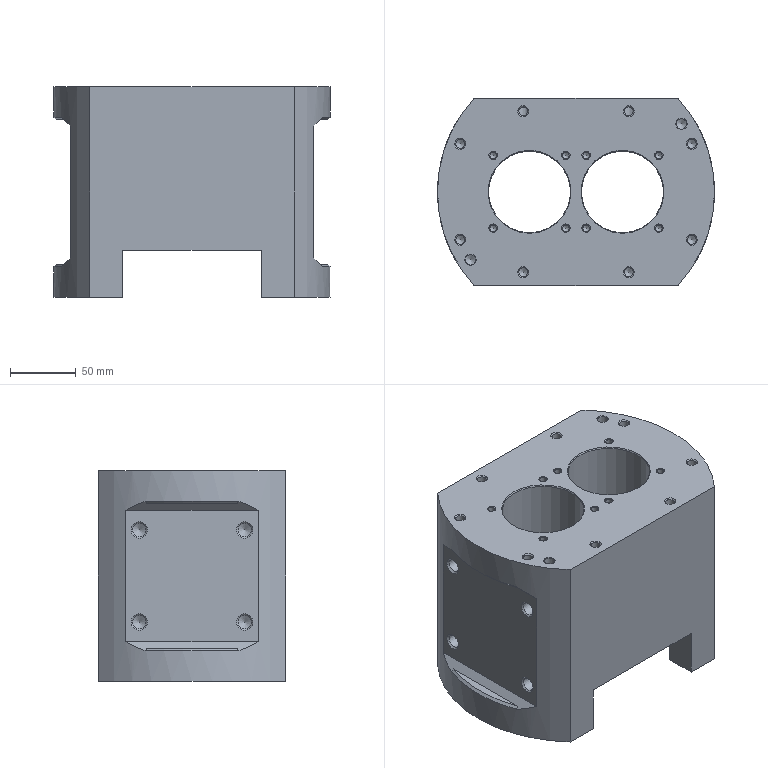NC program | NX | posted with a generic post | part box 210 x 142 x 160 mm
Lines 470 to 2119 of 4730, first 1534 of 1648 lines:
(ZLEVEL_PROFILE_COPY_COPY , TOOL : D10)
N932 T10 M6
N934 G54
N936 G17 G0 G90 X54.432 Y-32.868 B0. C0. S3500 M3
N938 G43 Z30. H10
N940 Z2.859
N942 G94 G1 Z-0.141 F1000.
N944 X55.511 Y-31.778
N946 G3 X55.764 Y-30.811 R1.
N948 G2 X51.879 Y-8.915 R121.943 F2200.
N950 X53.503 Y20.951 R111.959
N952 X55.764 Y30.811 R130.983
N954 G1 X55.765 Y30.984 Z-0.189
N956 X55.768 Y31.156 Z-0.236
N958 X55.772 Y31.328 Z-0.283
N960 G3 X53.364 Y20.951 R129.193
N962 G1 X53.281 Y20.505
N964 G3 X51.988 Y-11.59 R111.539
N966 X55.772 Y-31.328 R123.16
N968 G1 X55.773 Y-31.499 Z-0.33
N970 X55.776 Y-31.67 Z-0.377
N972 X55.78 Y-31.84 Z-0.424
N974 G2 X52.279 Y-15.115 R123.455
N976 X52.684 Y17.865 R110.827
N978 X55.78 Y31.84 R127.123
N980 G1 X55.781 Y32.011 Z-0.471
N982 X55.783 Y32.182 Z-0.519
N984 X55.787 Y32.352 Z-0.566
N986 G3 X53.085 Y20.951 R129.934
N988 X51.753 Y-12.035 R111.53
N990 X55.788 Y-32.352 R123.802
N992 G1 Y-32.521 Z-0.613
N994 X55.79 Y-32.69 Z-0.66
N996 X55.795 Y-32.858 Z-0.707
N998 G2 X51.882 Y-14.264 R125.341
N1000 G1 X51.666 Y-12.481
N1002 G2 X52.946 Y20.951 R111.309
N1004 G1 X53.031 Y21.396
N1006 X53.121 Y21.842
N1008 G2 X55.795 Y32.858 R131.028
N1010 G1 X55.797 Y33.025 Z-0.754
N1012 X55.8 Y33.19 Z-0.801
N1014 X55.804 Y33.356 Z-0.849
N1016 G3 X52.982 Y21.842 R131.167
N1018 G1 X52.893 Y21.396
N1020 X52.807 Y20.951
N1022 G3 X51.525 Y-12.481 R111.179
N1024 G1 X51.741 Y-14.264
N1026 G3 X55.804 Y-33.356 R125.503
N1028 G1 X55.807 Y-33.521 Z-0.896
N1030 X55.81 Y-33.686 Z-0.943
N1032 X55.814 Y-33.851 Z-0.99
N1034 G2 X51.657 Y-14.71 R127.282
N1036 X52.754 Y21.396 R111.065
N1038 G1 X52.843 Y21.842
N1040 G2 X55.814 Y33.851 R132.662
N1042 G1 X55.818 Y34.012 Z-1.037
N1044 X55.822 Y34.173 Z-1.084
N1046 X55.826 Y34.334 Z-1.131
N1048 G3 X52.705 Y21.842 R131.086
N1050 G1 X52.615 Y21.396
N1052 G3 X51.517 Y-14.71 R110.891
N1054 X55.826 Y-34.334 R126.821
N1056 G1 X55.831 Y-34.495 Z-1.179
N1058 X55.835 Y-34.656 Z-1.226
N1060 X55.841 Y-34.816 Z-1.273
N1062 G2 X51.377 Y-14.71 R126.454
N1064 X52.476 Y21.396 R110.775
N1066 G1 X52.566 Y21.842
N1068 G2 X55.841 Y34.816 R130.126
N1070 G1 X55.843 Y34.978 Z-1.32
N1072 X55.848 Y35.139 Z-1.367
N1074 X55.856 Y35.298 Z-1.414
N1076 G3 X52.427 Y21.842 R130.376
N1078 G1 X52.337 Y21.396
N1080 G3 X51.237 Y-14.71 R110.658
N1082 X55.856 Y-35.298 R126.434
N1084 G1 Y-35.459 Z-1.461
N1086 X55.86 Y-35.62 Z-1.508
N1088 X55.871 Y-35.778 Z-1.556
N1090 G2 X51.097 Y-14.71 R126.474
N1092 X52.027 Y20.505 R110.646
N1094 G1 X52.111 Y20.951
N1096 X52.198 Y21.396
N1098 X52.288 Y21.842
N1100 G2 X55.871 Y35.778 R131.039
N1102 G1 X55.872 Y35.939 Z-1.603
N1104 X55.877 Y36.098 Z-1.65
N1106 X55.888 Y36.255 Z-1.697
N1108 G3 X51.496 Y18.276 R129.399
N1110 X51.349 Y-17.385 R110.064
N1112 X55.888 Y-36.254 R129.287
N1114 G1 X55.875 Y-36.442 Z-1.768
N1116 X55.868 Y-36.628 Z-1.839
N1118 G2 X51.281 Y-17.83 R130.392
N1120 X49.981 Y-5.894 R114.798
N1122 X49.9 Y-3.019 R51.159
N1124 G1 Y2.816
N1126 G2 X50.036 Y6.901 R61.241
N1128 X53.454 Y28.22 R117.257
N1130 G1 X53.566 Y28.655
N1132 G2 X55.868 Y36.629 R138.665
N1134 G1 X55.801 Y36.638 Z-1.909
N1136 X55.709 Y36.651 Z-1.98
N1138 X55.636 Y36.329
N1140 G3 X53.174 Y27.657 R143.814
N1142 X50.01 Y8.459 R118.727
N1144 X49.9 Y6.104 R34.256
N1146 G1 Y-6.102
N1148 G3 X50.011 Y-8.469 R34.223
N1150 X51.069 Y-17.385 R117.376
N1152 X55.289 Y-35.215 R128.669
N1154 G1 X55.653 Y-36.391
N1156 G2 X55.711 Y-36.653 R1.619
N1158 G1 X55.607 Y-36.717 Z-2.051
N1160 X55.524 Y-36.779 Z-2.122
N1162 G3 X55.381 Y-35.942 R3.116
N1164 G1 X55.292 Y-35.661
N1166 G2 X51.003 Y-17.83 R129.053
N1168 X49.949 Y-9.361 R112.033
N1170 X49.9 Y-8.147 R16.629
N1172 G1 Y8.25
N1174 G2 X49.949 Y9.361 R12.69
N1176 X53.488 Y29.42 R117.251
N1178 X55.386 Y35.965 R152.215
N1180 G3 X55.513 Y36.782 R2.769
N1182 G1 X55.435 Y36.945 Z-2.193
N1184 X55.364 Y37.108 Z-2.264
N1186 G2 X55.295 Y36.106 R10.2
N1188 G1 X54.216 Y32.54
N1190 X54.088 Y32.095
N1192 G3 X50.017 Y11.59 R120.931
N1194 X49.9 Y9.784 R18.15
N1196 G1 Y-9.778
N1198 G3 X50.017 Y-11.59 R18.112
N1200 X50.789 Y-17.385 R128.232
N1202 X55.298 Y-36.106 R129.171
N1204 G2 X55.365 Y-37.108 R18.347
N1206 G1 X55.283 Y-37.269 Z-2.336
N1208 X55.209 Y-37.431 Z-2.407
N1210 X55.183 Y-36.329
N1212 X55.162 Y-36.106
N1214 G2 X50.648 Y-17.385 R129.228
N1216 X49.984 Y-12.497 R91.731
N1218 X49.9 Y-11.159 R14.702
N1220 G1 Y11.159
N1222 G2 X49.982 Y12.481 R14.7
N1224 G1 X50.035 Y12.927
N1226 G2 X52.969 Y28.487 R116.607
N1228 X55.159 Y36.106 R155.692
N1230 G1 X55.187 Y36.329
N1232 X55.208 Y37.431
N1234 X55.132 Y37.585 Z-2.478
N1236 X55.068 Y37.738 Z-2.549
N1238 X55.044 Y36.329
N1240 X55.023 Y36.106
N1242 X53.944 Y32.54
N1244 X53.815 Y32.095
N1246 G3 X50.053 Y14.264 R122.42
N1248 X49.9 Y12.412 R16.173
N1250 G1 Y-12.412
N1252 G3 X50.053 Y-14.264 R16.169
N1254 X51.05 Y-20.505 R128.494
N1256 X55.027 Y-36.106 R132.286
N1258 G1 X55.066 Y-37.739
N1260 X54.985 Y-37.895 Z-2.62
N1262 X54.918 Y-38.051 Z-2.691
N1264 X54.912 Y-37.889
N1266 X54.893 Y-36.329
N1268 X54.888 Y-36.106
N1270 G2 X50.911 Y-20.505 R132.995
N1272 X49.958 Y-14.562 R100.549
N1274 X49.9 Y-13.672 R6.915
N1276 G1 Y13.532
N1278 G2 X49.977 Y14.71 R8.722
N1280 X53.808 Y32.54 R121.32
N1282 G1 X53.939 Y32.986
N1284 X54.886 Y36.106
N1286 X54.902 Y36.329
N1288 X54.913 Y37.889
N1290 X54.918 Y38.051
N1292 X54.844 Y38.218 Z-2.762
N1294 X54.775 Y38.385 Z-2.833
N1296 X54.773 Y38.335
N1298 X54.761 Y36.329
N1300 X54.749 Y36.106
N1302 X53.542 Y32.095
N1304 G3 X50.159 Y16.939 R123.062
N1306 G1 X50.029 Y16.047
N1308 G3 X49.9 Y14.567 R11.273
N1310 G1 Y-14.563
N1312 G3 X50.029 Y-16.047 R11.25
N1314 G1 X50.159 Y-16.939
N1316 G3 X53.99 Y-33.6 R122.929
N1318 G1 X54.618 Y-35.661
N1320 X54.745 Y-36.106
N1322 X54.749 Y-36.329
N1324 X54.774 Y-38.385
N1326 X54.702 Y-38.577 Z-2.904
N1328 X54.632 Y-38.769 Z-2.975
N1330 X54.631 Y-38.335
N1332 X54.602 Y-36.106
N1334 X54.504 Y-35.74
N1336 X53.8 Y-33.432
N1338 G2 X50.089 Y-17.385 R124.615
N1340 G1 X50.019 Y-16.939
N1342 G2 X49.9 Y-15.522 R10.96
N1344 G1 Y15.525
N1346 G2 X50.019 Y16.939 R10.975
N1348 X53.577 Y32.681 R121.322
N1350 G1 X53.801 Y33.432
N1352 X54.48 Y35.661
N1354 X54.611 Y36.106
N1356 X54.619 Y36.329
N1358 X54.632 Y38.335
N1360 X54.633 Y38.768
N1362 X54.562 Y38.96 Z-3.045
N1364 X54.492 Y39.152 Z-3.116
N1366 X54.491 Y38.781
N1368 X54.478 Y36.329
N1370 X54.472 Y36.106
N1372 X54.345 Y35.661
N1374 X53.666 Y33.432
N1376 G3 X50.027 Y17.83 R123.198
N1378 X49.9 Y16.425 R8.144
N1380 G1 Y-16.426
N1382 G3 X50.008 Y-17.723 R8.144
N1384 X53.786 Y-33.831 R123.596
N1386 G1 X54.352 Y-35.678
N1388 G2 X54.459 Y-36.106 R4.153
N1390 G1 X54.492 Y-39.152
N1392 X54.421 Y-39.339 Z-3.187
N1394 X54.355 Y-39.526 Z-3.257
N1396 X54.315 Y-36.106
N1398 G3 X54.19 Y-35.584 R4.242
N1400 G1 X53.693 Y-33.97
N1402 G2 X50.03 Y-18.661 R123.344
N1404 X49.9 Y-17.282 R8.987
N1406 G1 Y17.279
N1408 G2 X50.041 Y18.722 R8.981
N1410 X53.531 Y33.432 R122.706
N1412 G1 X54.211 Y35.661
N1414 X54.329 Y36.106
N1416 X54.335 Y36.329
N1418 X54.355 Y39.526
N1420 X54.28 Y39.712 Z-3.328
N1422 X54.214 Y39.897 Z-3.399
N1424 X54.197 Y36.552
N1426 X54.186 Y36.106
N1428 G2 X54.039 Y35.54 R6.808
N1430 G1 X53.621 Y34.167
N1432 G3 X50.054 Y19.613 R124.947
N1434 X49.9 Y18.07 R8.694
N1436 G1 Y-18.073
N1438 G3 X50.013 Y-19.374 R7.569
N1440 G1 X50.132 Y-20.059
N1442 G3 X53.561 Y-33.977 R126.794
N1444 G1 X54.059 Y-35.599
N1446 G2 X54.171 Y-36.106 R3.232
N1448 X54.214 Y-39.898 R175.48
N1450 G1 X54.138 Y-40.083 Z-3.47
N1452 X54.071 Y-40.268 Z-3.54
N1454 G3 X54.01 Y-35.884 R87.583
N1456 G2 X50.028 Y-20.231 R133.069
N1458 X49.9 Y-18.874 R7.249
N1460 G1 Y18.869
N1462 G2 X50.045 Y20.342 R8.152
N1464 X53.807 Y35.215 R129.906
N1466 G1 X54.01 Y35.884
N1468 X54.042 Y36.106
N1470 X54.056 Y36.552
N1472 X54.071 Y40.268
N1474 X53.997 Y40.452 Z-3.611
N1476 X53.93 Y40.637 Z-3.682
N1478 X53.918 Y36.998
N1480 X53.898 Y36.045
N1482 X53.899 Y35.947
N1484 X53.867 Y35.854
N1486 X53.673 Y35.215
N1488 G3 X50.089 Y21.246 R126.418
N1490 G1 X50.032 Y20.951
N1492 G3 X49.9 Y19.613 R7.981
N1494 G1 Y-19.613
N1496 G3 X50.058 Y-21.089 R8.1
N1498 G1 X50.478 Y-23.179
N1500 G3 X53.874 Y-35.884 R137.422
N1502 G2 X53.93 Y-40.637 R126.919
N1504 G1 X53.856 Y-40.817 Z-3.752
N1506 X53.786 Y-40.998 Z-3.823
N1508 G3 X53.738 Y-35.884 R149.866
N1510 G2 X51.27 Y-27.191 R149.045
N1512 X50.03 Y-21.645 R109.625
N1514 X49.9 Y-20.312 R6.909
N1516 G1 Y20.311
N1518 G2 X50.041 Y21.693 R7.571
N1520 G1 X50.089 Y21.946
N1522 X50.157 Y22.288
N1524 G2 X53.7 Y35.742 R131.324
N1526 G3 X53.755 Y36.065 R1.143
N1528 G1 X53.776 Y36.998
N1530 X53.786 Y40.998
N1532 X53.715 Y41.176 Z-3.894
N1534 X53.646 Y41.354 Z-3.965
N1536 X53.627 Y36.552
N1538 X53.606 Y35.884
N1540 X52.992 Y33.878
N1542 G3 X50.089 Y22.646 R126.885
N1544 X49.9 Y21.024 R8.181
N1546 G1 Y-21.025
N1548 G3 X50.107 Y-22.734 R8.449
N1550 X53.602 Y-35.884 R137.683
N1552 G2 X53.646 Y-41.354 R180.795
N1554 G1 X53.573 Y-41.532 Z-4.035
N1556 X53.507 Y-41.709 Z-4.106
N1558 X53.488 Y-36.998
N1560 X53.464 Y-35.884
N1562 G2 X51.957 Y-30.812 R200.511
N1564 X50.042 Y-23.06 R119.172
N1566 X49.9 Y-21.705 R6.544
N1568 G1 Y21.694
N1570 G2 X50.048 Y23.089 R6.661
N1572 X53.271 Y35.215 R128.308
N1574 G1 X53.465 Y35.884
N1576 X53.494 Y36.998
N1578 X53.507 Y41.709
N1580 X53.432 Y41.886 Z-4.177
N1582 X53.365 Y42.062 Z-4.247
N1584 X53.352 Y36.998
N1586 X53.325 Y35.884
N1588 G2 X53.153 Y35.264 R8.232
N1590 G3 X50.089 Y23.899 R126.068
N1592 X49.9 Y22.343 R7.417
N1594 G1 Y-22.34
N1596 G3 X50.089 Y-23.899 R7.414
N1598 X52.316 Y-32.54 R122.93
N1600 G1 X52.448 Y-32.986
N1602 X53.268 Y-35.661
N1604 X53.326 Y-35.884
N1606 X53.348 Y-36.998
N1608 X53.365 Y-42.062
N1610 X53.29 Y-42.236 Z-4.318
N1612 X53.222 Y-42.411 Z-4.389
N1614 X53.209 Y-36.998
N1616 X53.179 Y-35.832
N1618 G2 X51.062 Y-28.529 R168.762
N1620 X50.064 Y-24.401 R94.596
N1622 X49.9 Y-22.94 R7.131
N1624 G1 Y22.939
N1626 G2 X50.089 Y24.515 R7.13
N1628 X53.003 Y35.215 R126.159
N1630 G1 X53.179 Y35.834
N1632 X53.185 Y35.884
N1634 X53.21 Y36.998
N1636 X53.222 Y42.411
N1638 X53.149 Y42.582 Z-4.46
N1640 X53.079 Y42.753 Z-4.53
N1642 X53.07 Y36.998
N1644 X53.049 Y36.02
N1646 G2 X52.963 Y35.509 R1.789
N1648 G3 X50.089 Y25.13 R128.441
N1650 X49.9 Y23.58 R7.428
N1652 G1 Y-23.583
N1654 G3 X50.111 Y-25.236 R8.012
N1656 X52.889 Y-35.302 R136.594
N1658 G2 X53.051 Y-35.884 R8.688
N1660 G1 X53.062 Y-36.552
N1662 X53.079 Y-42.753
N1664 X53.008 Y-42.924 Z-4.601
N1666 X52.943 Y-43.095 Z-4.672
N1668 X52.937 Y-42.793
N1670 X52.93 Y-36.998
N1672 X52.915 Y-35.884
N1674 G3 X52.785 Y-35.398 R5.308
N1676 G2 X50.12 Y-25.854 R137.329
N1678 G1 X50.089 Y-25.725
N1680 G2 X49.9 Y-24.176 R6.808
N1682 G1 Y24.176
N1684 G2 X50.089 Y25.725 R6.808
N1686 G1 X50.12 Y25.854
N1688 G2 X52.871 Y35.661 R136.201
N1690 G3 X52.911 Y35.968 R1.414
N1692 G1 X52.929 Y36.998
N1694 X52.937 Y42.793
N1696 X52.943 Y43.095
N1698 X52.866 Y43.266 Z-4.742
N1700 X52.8 Y43.437 Z-4.813
N1702 X52.789 Y36.998
N1704 X52.774 Y35.972
N1706 G2 X52.738 Y35.663 R1.498
N1708 G3 X50.089 Y26.28 R133.364
N1710 X49.9 Y24.758 R6.314
N1712 G1 Y-24.755
N1714 G3 X50.08 Y-26.243 R6.314
N1716 X52.7 Y-35.534 R137.19
N1718 G2 X52.788 Y-36.093 R1.843
N1720 G1 X52.8 Y-43.437
N1722 X52.725 Y-43.604 Z-4.884
N1724 X52.657 Y-43.771 Z-4.955
N1726 X52.649 Y-36.552
N1728 X52.642 Y-35.989
N1730 G3 X52.572 Y-35.563 R1.447
N1732 G2 X50.089 Y-26.828 R130.266
N1734 X49.9 Y-25.321 R6.298
N1736 G1 Y25.321
N1738 G2 X50.089 Y26.828 R6.298
N1740 X52.604 Y35.661 R130.864
N1742 G3 X52.641 Y36.123 R3.131
N1744 G1 X52.652 Y37.889
N1746 X52.654 Y43.684
N1748 X52.657 Y43.771
N1750 X52.583 Y43.936 Z-5.025
N1752 X52.514 Y44.1 Z-5.096
N1754 X52.511 Y37.889
N1756 X52.503 Y36.181
N1758 G2 X52.47 Y35.661 R4.448
N1760 G3 X50.089 Y27.376 R132.336
N1762 X49.9 Y25.854 R6.358
N1764 G1 Y-25.854
N1766 G3 X50.089 Y-27.376 R6.359
N1768 X52.432 Y-35.542 R130.045
N1770 G2 X52.504 Y-35.986 R1.481
N1772 G1 X52.508 Y-36.552
N1774 X52.514 Y-44.1
N1776 X52.442 Y-44.265 Z-5.167
N1778 X52.375 Y-44.429 Z-5.237
N1780 X52.371 Y-44.13
N1782 X52.37 Y-37.444
N1784 X52.366 Y-35.884
N1786 G3 X52.266 Y-35.439 R2.557
N1788 G2 X50.129 Y-28.083 R137.56
N1790 X49.9 Y-26.414 R6.579
N1792 G1 Y26.414
N1794 G2 X50.129 Y28.083 R6.579
N1796 X52.336 Y35.661 R140.237
N1798 G1 X52.366 Y36.552
N1800 X52.37 Y37.889
N1802 X52.371 Y44.13
N1804 X52.375 Y44.429
N1806 X52.301 Y44.594 Z-5.308
N1808 X52.234 Y44.758 Z-5.379
N1810 X52.226 Y36.998
N1812 X52.202 Y35.661
N1814 G3 X50.108 Y28.529 R143.996
N1816 X49.9 Y26.942 R6.229
N1818 G1 Y-26.942
N1820 G3 X50.089 Y-28.458 R6.228
N1822 X52.171 Y-35.56 R139.376
N1824 G2 X52.227 Y-35.911 R1.15
N1826 G1 X52.229 Y-37.444
N1828 X52.23 Y-44.576
N1830 X52.234 Y-44.758
N1832 X52.159 Y-44.921 Z-5.449
N1834 X52.09 Y-45.083 Z-5.52
N1836 X52.088 Y-45.022
N1838 Y-37.444
N1840 X52.085 Y-35.742
N1842 G2 X50.089 Y-28.956 R156.875
N1844 X49.9 Y-27.46 R6.103
N1846 G1 Y27.459
N1848 G2 X50.089 Y28.956 R6.104
N1850 X52.067 Y35.661 R139.109
N1852 G1 X52.085 Y36.552
N1854 X52.09 Y45.083
N1856 X52.018 Y45.242 Z-5.591
N1858 X51.949 Y45.401 Z-5.662
N1860 X51.941 Y36.106
N1862 X51.931 Y35.661
N1864 G3 X50.089 Y29.45 R137.86
N1866 X49.9 Y27.968 R6.103
N1868 G1 Y-27.968
N1870 G3 X50.089 Y-29.45 R6.103
N1872 X51.936 Y-35.661 R129.992
N1874 G1 X51.945 Y-35.771
N1876 X51.949 Y-45.401
N1878 X51.876 Y-45.559 Z-5.732
N1880 X51.809 Y-45.718 Z-5.803
N1882 X51.806 Y-45.467
N1884 X51.805 Y-36.552
N1886 X51.803 Y-35.661
N1888 G2 X50.108 Y-30.011 R126.75
N1890 X49.9 Y-28.469 R5.822
N1892 G1 Y28.465
N1894 G2 X50.112 Y30.024 R5.843
N1896 X51.795 Y35.661 R145.292
N1898 G1 X51.803 Y36.106
N1900 X51.806 Y45.467
N1902 X51.809 Y45.718
N1904 X51.735 Y45.876 Z-5.874
N1906 X51.67 Y46.035 Z-5.944
N1908 X51.658 Y35.661
N1910 G3 X50.177 Y30.757 R208.31
N1912 X49.9 Y28.951 R6.443
N1914 G1 Y-28.953
N1916 G3 X50.177 Y-30.757 R6.443
N1918 X51.663 Y-35.661 R170.484
N1920 G1 X51.664 Y-45.913
N1922 X51.67 Y-46.035
N1924 X51.593 Y-46.194 Z-6.015
N1926 X51.523 Y-46.352 Z-6.086
N1928 X51.522 Y-35.661
N1930 G2 X50.169 Y-31.203 R391.393
N1932 X49.9 Y-29.42 R6.165
N1934 G1 Y29.426
N1936 G2 X50.129 Y31.064 R5.973
N1938 G1 X50.169 Y31.203
N1940 X50.969 Y33.878
N1942 X51.491 Y35.555
N1944 X51.52 Y35.661
N1946 X51.522 Y36.106
N1948 X51.523 Y46.352
N1950 X51.452 Y46.505 Z-6.157
N1952 X51.383 Y46.658 Z-6.227
N1954 X51.381 Y46.359
N1956 Y35.6
N1958 G3 X50.133 Y31.538 R147.034
N1960 X49.9 Y29.903 R5.843
N1962 G1 Y-29.903
N1964 G3 X50.133 Y-31.538 R5.843
N1966 X51.381 Y-35.6 R147.008
N1968 G1 Y-46.359
N1970 X51.383 Y-46.658
N1972 X51.311 Y-46.811 Z-6.298
N1974 X51.246 Y-46.964 Z-6.369
N1976 X51.24 Y-46.805
N1978 Y-35.575
N1980 G2 X50.129 Y-31.971 R120.925
N1982 X49.9 Y-30.368 R5.731
N1984 G1 Y30.368
N1986 G2 X50.129 Y31.971 R5.732
N1988 X51.24 Y35.575 R120.9
N1990 G1 Y46.805
N1992 X51.246 Y46.964
N1994 X51.169 Y47.117 Z-6.439
N1996 X51.099 Y47.27 Z-6.51
N1998 X51.098 Y36.586
N2000 Y35.55
N2002 G3 X50.129 Y32.419 R104.477
N2004 X49.9 Y30.823 R5.684
N2006 G1 Y-30.822
N2008 G3 X50.129 Y-32.419 R5.685
N2010 X51.098 Y-35.55 R104.477
N2012 G1 Y-36.587
N2014 X51.099 Y-47.27
N2016 X51.028 Y-47.423 Z-6.581
N2018 X50.958 Y-47.576 Z-6.652
N2020 X50.957 Y-36.965
N2022 Y-35.525
N2024 G2 X50.131 Y-32.875 R89.581
N2026 X49.9 Y-31.272 R5.672
N2028 G1 Y31.272
N2030 G2 X50.131 Y32.875 R5.673
N2032 X50.957 Y35.525 R89.581
N2034 G1 Y47.25
N2036 X50.958 Y47.576
N2038 X50.886 Y47.726 Z-6.722
N2040 X50.821 Y47.875 Z-6.793
N2042 X50.816 Y47.696
N2044 Y35.5
N2046 X50.159 Y33.403
N2048 G3 X49.9 Y31.71 R5.665
N2050 G1 Y-31.719
N2052 G3 X50.156 Y-33.394 R5.608
N2054 G1 X50.816 Y-35.5
N2056 Y-47.696
N2058 X50.821 Y-47.875
N2060 X50.745 Y-48.024 Z-6.864
N2062 X50.675 Y-48.172 Z-6.934
N2064 X50.674 Y-37.444
N2066 Y-35.465
N2068 X50.168 Y-33.878
N2070 X50.153 Y-33.826
N2072 G2 X49.9 Y-32.146 R5.713
N2074 G1 Y32.146
N2076 G2 X50.153 Y33.826 R5.713
N2078 G1 X50.168 Y33.878
N2080 X50.674 Y35.465
N2082 Y37.444
N2084 X50.675 Y48.172
N2086 X50.603 Y48.319 Z-7.005
N2088 X50.534 Y48.467 Z-7.076
N2090 X50.533 Y38.075
N2092 X50.532 Y35.439
N2094 X50.163 Y34.275
N2096 G3 X49.9 Y32.576 R5.623
N2098 G1 Y-32.576
N2100 G3 X50.163 Y-34.275 R5.623
N2102 G1 X50.532 Y-35.439
N2104 X50.533 Y-38.075
N2106 X50.534 Y-48.467
N2108 X50.462 Y-48.614 Z-7.147
N2110 X50.397 Y-48.762 Z-7.217
N2112 X50.391 Y-48.588
N2114 Y-38.335
N2116 Y-35.406
N2118 X50.162 Y-34.684
N2120 G2 X49.9 Y-32.993 R5.594
N2122 G1 Y32.993
N2124 G2 X50.162 Y34.684 R5.594
N2126 G1 X50.391 Y35.406
N2128 Y38.335
N2130 Y48.588
N2132 X50.397 Y48.762
N2134 X50.321 Y48.909 Z-7.288
N2136 X50.251 Y49.056 Z-7.359
N2138 X50.25 Y38.781
N2140 Y35.394
N2142 G3 X49.9 Y33.41 R6.074
N2144 G1 Y-33.411
N2146 G3 X50.25 Y-35.394 R6.075
N2148 G1 Y-38.781
N2150 X50.251 Y-49.056
N2152 X50.179 Y-49.2 Z-7.429
N2154 X50.111 Y-49.344 Z-7.5
N2156 X50.108 Y-38.781
N2158 Y-35.361
N2160 G2 X49.9 Y-33.823 R6.105
N2162 G1 Y33.822
N2164 G2 X50.108 Y35.361 R6.104
N2166 G1 Y38.781
N2168 X50.111 Y49.344
N2170 X50.038 Y49.486 Z-7.571
N2172 X49.972 Y49.629 Z-7.642
N2174 X49.967 Y49.479
N2176 Y35.18
N2178 G3 X49.9 Y34.226 R11.448
N2180 G1 Y-34.226
N2182 G3 X49.967 Y-35.18 R11.461
N2184 G1 Y-49.479
N2186 X49.972 Y-49.629
N2188 X49.896 Y-49.772 Z-7.712
N2190 X49.826 Y-49.914 Z-7.783
N2192 Y-39.672
N2194 Y39.672
N2196 Y49.914
N2198 X49.755 Y50.057 Z-7.854
N2200 X49.687 Y50.199 Z-7.924
N2202 X49.684 Y49.925
N2204 Y-49.925
N2206 X49.687 Y-50.199
N2208 X49.613 Y-50.34 Z-7.995
N2210 X49.547 Y-50.481 Z-8.066
N2212 X49.543 Y-50.371
N2214 X49.541 Y-40.529
N2216 X49.543 Y-40.118
N2218 Y40.118
N2220 X49.541 Y40.529
N2222 X49.543 Y50.371
N2224 X49.547 Y50.481
N2226 X49.472 Y50.62 Z-8.137
N2228 X49.404 Y50.759 Z-8.207
N2230 X49.401 Y50.371
N2232 Y-50.371
N2234 X49.404 Y-50.759
N2236 X49.331 Y-50.897 Z-8.278
N2238 X49.264 Y-51.035 Z-8.349
N2240 X49.26 Y-50.816
N2242 Y50.816
N2244 X49.264 Y51.035
N2246 X49.189 Y51.172 Z-8.419
N2248 X49.121 Y51.31 Z-8.49
N2250 X49.119 Y41.456
N2252 Y-41.456
N2254 X49.121 Y-51.31
N2256 X49.048 Y-51.448 Z-8.561
N2258 X48.982 Y-51.585 Z-8.631
N2260 X48.977 Y-51.262
N2262 X48.976 Y-41.855
N2264 X48.977 Y-41.456
N2266 Y41.456
N2268 X48.976 Y41.855
N2270 X48.977 Y51.262
N2272 X48.982 Y51.585
N2274 X48.906 Y51.722 Z-8.702
N2276 X48.84 Y51.858 Z-8.773
N2278 X48.836 Y51.708
N2280 Y-51.708
N2282 X48.84 Y-51.858
N2284 X48.765 Y-51.992 Z-8.844
N2286 X48.695 Y-52.127 Z-8.914
N2288 X48.694 Y-42.347
N2290 Y42.347
N2292 X48.695 Y52.127
N2294 X48.624 Y52.26 Z-8.985
N2296 X48.559 Y52.393 Z-9.056
N2298 X48.553 Y52.154
N2300 Y-52.154
N2302 X48.559 Y-52.393
N2304 X48.482 Y-52.526 Z-9.126
N2306 X48.414 Y-52.659 Z-9.197
N2308 X48.411 Y-42.793
N2310 Y42.793
N2312 X48.414 Y52.659
N2314 X48.341 Y52.792 Z-9.268
N2316 X48.272 Y52.925 Z-9.339
N2318 X48.27 Y52.599
N2320 Y-52.599
N2322 X48.272 Y-52.925
N2324 X48.199 Y-53.058 Z-9.409
N2326 X48.134 Y-53.19 Z-9.48
N2328 X48.129 Y-53.045
N2330 Y53.045
N2332 X48.134 Y53.19
N2334 X48.058 Y53.322 Z-9.551
N2336 X47.989 Y53.454 Z-9.621
N2338 X47.987 Y43.684
N2340 Y-43.684
N2342 X47.989 Y-53.454
N2344 X47.916 Y-53.585 Z-9.692
N2346 X47.849 Y-53.716 Z-9.763
N2348 X47.846 Y-53.491
N2350 Y53.491
N2352 X47.849 Y53.716
N2354 X47.775 Y53.847 Z-9.834
N2356 X47.707 Y53.978 Z-9.904
N2358 X47.704 Y53.937
N2360 Y-53.937
N2362 X47.707 Y-53.978
N2364 X47.634 Y-54.11 Z-9.975
N2366 X47.569 Y-54.241 Z-10.046
N2368 X47.563 Y-53.937
N2370 Y53.937
N2372 X47.569 Y54.241
N2374 X47.492 Y54.372 Z-10.116
N2376 X47.424 Y54.503 Z-10.187
N2378 X47.421 Y54.383
N2380 Y-54.383
N2382 X47.424 Y-54.503
N2384 X47.351 Y-54.635 Z-10.258
N2386 X47.282 Y-54.766 Z-10.329
N2388 X47.28 Y-45.467
N2390 Y45.467
N2392 X47.282 Y54.766
N2394 X47.209 Y54.897 Z-10.399
N2396 X47.143 Y55.028 Z-10.47
N2398 X47.139 Y54.828
N2400 Y-54.828
N2402 X47.143 Y-55.028
N2404 X47.068 Y-55.159 Z-10.541
N2406 X46.998 Y-55.291 Z-10.611
N2408 X46.997 Y-46.143
N2410 Y46.143
N2412 X46.998 Y55.291
N2414 X46.926 Y55.422 Z-10.682
N2416 X46.86 Y55.553 Z-10.753
N2418 X46.856 Y55.274
N2420 Y-55.274
N2422 X46.86 Y-55.553
N2424 X46.785 Y-55.684 Z-10.824
N2426 X46.717 Y-55.815 Z-10.894
N2428 X46.714 Y-55.72
N2430 Y55.72
N2432 X46.717 Y55.815
N2434 X46.644 Y55.947 Z-10.965
N2436 X46.574 Y56.078 Z-11.036
N2438 X46.573 Y46.805
N2440 Y-46.805
N2442 X46.574 Y-56.078
N2444 X46.502 Y-56.209 Z-11.106
N2446 X46.436 Y-56.34 Z-11.177
N2448 X46.432 Y-56.166
N2450 Y56.166
N2452 X46.436 Y56.34
N2454 X46.361 Y56.471 Z-11.248
N2456 X46.29 Y56.602 Z-11.318
N2458 Y47.25
N2460 Y-47.25
N2462 Y-56.602
N2464 X46.219 Y-56.734 Z-11.389
N2466 X46.152 Y-56.865 Z-11.46
N2468 X46.149 Y-56.611
N2470 Y56.611
N2472 X46.152 Y56.865
N2474 X46.078 Y56.996 Z-11.531
N2476 X46.01 Y57.127 Z-11.601
N2478 X46.007 Y57.057
N2480 Y-57.057
N2482 X46.01 Y-57.127
N2484 X45.937 Y-57.258 Z-11.672
N2486 X45.87 Y-57.39 Z-11.743
N2488 X45.866 Y-57.057
N2490 Y57.057
N2492 X45.87 Y57.39
N2494 X45.795 Y57.521 Z-11.813
N2496 X45.728 Y57.652 Z-11.884
N2498 X45.724 Y57.503
N2500 Y-57.503
N2502 X45.728 Y-57.652
N2504 X45.654 Y-57.783 Z-11.955
N2506 X45.584 Y-57.914 Z-12.026
N2508 X45.583 Y-48.588
N2510 Y48.588
N2512 X45.584 Y57.914
N2514 X45.512 Y58.046 Z-12.096
N2516 X45.448 Y58.177 Z-12.167
N2518 X45.442 Y57.949
N2520 Y-57.949
N2522 X45.448 Y-58.177
N2524 X45.381 Y-58.289 Z-12.227
N2526 X45.321 Y-58.401 Z-12.288
N2528 Y-49.033
N2530 Y49.033
N2532 Y58.401
N2534 X45.26 Y58.513 Z-12.348
N2536 X45.203 Y58.625 Z-12.409
N2538 X45.2 Y58.394
N2540 Y-58.394
N2542 X45.203 Y-58.625
N2544 X45.14 Y-58.737 Z-12.469
N2546 X45.08 Y-58.849 Z-12.529
N2548 X45.079 Y-49.872
N2550 Y49.872
N2552 X45.08 Y58.849
N2554 X45.019 Y58.959 Z-12.59
N2556 X44.968 Y59.068 Z-12.65
N2558 X44.961 Y58.84
N2560 Y-58.84
N2562 X44.968 Y-59.068
N2564 G2 X44.495 Y-59.949 R1.
N2566 G1 X43.17 Y-60.769
N2568 Z-9.65
N2570 G0 Z30.
N2572 X-54.433 Y32.867
N2574 Z2.859
N2576 G1 Z-0.141 F1000.
N2578 X-55.511 Y31.778
N2580 G3 X-55.765 Y30.811 R1.
N2582 G2 X-51.879 Y8.915 R121.826 F2200.
N2584 X-53.42 Y-20.505 R111.854
N2586 G1 X-53.503 Y-20.951
N2588 G2 X-55.765 Y-30.811 R129.768
N2590 G1 Y-30.984 Z-0.189
N2592 X-55.768 Y-31.156 Z-0.236
N2594 X-55.774 Y-31.327 Z-0.283
N2596 G3 X-53.364 Y-20.951 R127.93
N2598 G1 X-53.281 Y-20.505
N2600 G3 X-51.988 Y11.59 R111.539
N2602 X-55.774 Y31.328 R122.8
N2604 G1 X-55.773 Y31.499 Z-0.33
N2606 X-55.776 Y31.67 Z-0.377
N2608 X-55.782 Y31.839 Z-0.424
N2610 G2 X-51.847 Y11.59 R122.699
N2612 X-53.309 Y-21.396 R111.821
N2614 G1 X-53.398 Y-21.842
N2616 G2 X-55.782 Y-31.839 R125.448
N2618 G1 X-55.781 Y-32.011 Z-0.471
N2620 X-55.783 Y-32.182 Z-0.519
N2622 X-55.79 Y-32.351 Z-0.566
N2624 G3 X-52.581 Y-18.09 R127.234
N2626 X-52.152 Y15.21 R110.749
N2628 X-55.79 Y32.351 R123.427
N2630 G1 X-55.788 Y32.521 Z-0.613
N2632 X-55.79 Y32.69 Z-0.66
N2634 X-55.797 Y32.858 Z-0.707
N2636 G2 X-51.613 Y12.035 R123.979
N2638 X-53.031 Y-21.396 R111.521
N2640 G1 X-53.121 Y-21.842
N2642 G2 X-55.797 Y-32.858 R129.545
N2644 G1 Y-33.025 Z-0.754
N2646 X-55.8 Y-33.19 Z-0.801
N2648 X-55.805 Y-33.355 Z-0.849
N2650 G3 X-52.982 Y-21.842 R130.582
N2652 G1 X-52.893 Y-21.396
N2654 G3 X-51.741 Y14.264 R111.099
N2656 X-55.805 Y33.355 R125.466
N2658 G1 X-55.807 Y33.521 Z-0.896
N2660 X-55.81 Y33.686 Z-0.943
N2662 X-55.814 Y33.851 Z-0.99
N2664 G2 X-51.657 Y14.71 R126.853
N2666 X-52.754 Y-21.396 R111.038
N2668 G1 X-52.843 Y-21.842
N2670 G2 X-55.814 Y-33.85 R132.144
N2672 G1 X-55.818 Y-34.012 Z-1.037
N2674 X-55.822 Y-34.173 Z-1.084
N2676 X-55.827 Y-34.334 Z-1.131
N2678 G3 X-52.705 Y-21.842 R131.047
N2680 G1 X-52.615 Y-21.396
N2682 G3 X-51.517 Y14.71 R110.89
N2684 X-55.827 Y34.334 R126.796
N2686 G1 X-55.831 Y34.495 Z-1.179
N2688 X-55.835 Y34.656 Z-1.226
N2690 X-55.84 Y34.817 Z-1.273
N2692 G2 X-51.377 Y14.71 R126.672
N2694 X-52.476 Y-21.396 R110.771
N2696 G1 X-52.566 Y-21.842
N2698 G2 X-55.84 Y-34.817 R130.863
N2700 G1 X-55.843 Y-34.978 Z-1.32
N2702 X-55.848 Y-35.139 Z-1.367
N2704 X-55.853 Y-35.299 Z-1.414
N2706 G3 X-52.427 Y-21.842 R131.577
N2708 G1 X-52.337 Y-21.396
N2710 G3 X-51.237 Y14.71 R110.652
N2712 X-55.853 Y35.299 R126.944
N2714 G1 X-55.856 Y35.46 Z-1.461
N2716 X-55.861 Y35.62 Z-1.508
N2718 X-55.867 Y35.779 Z-1.556
N2720 G2 X-51.56 Y17.83 R130.114
N2722 X-52.288 Y-21.842 R110.567
N2724 X-55.867 Y-35.78 R133.324
N2726 G1 X-55.872 Y-35.939 Z-1.603
N2728 X-55.877 Y-36.098 Z-1.65
N2730 X-55.883 Y-36.257 Z-1.697
N2732 G3 X-52.149 Y-21.842 R133.61
N2734 X-51.421 Y17.83 R110.456
N2736 X-55.883 Y36.256 R130.454
N2738 G1 X-55.886 Y36.476 Z-1.768
N2740 X-55.888 Y36.695 Z-1.839
N2742 G2 X-51.282 Y17.83 R130.949
N2744 X-49.975 Y5.795 R114.769
N2746 X-49.9 Y2.809 R69.546
N2748 G1 Y-2.847
N2750 G2 X-50.02 Y-6.468 R54.717
N2752 G1 X-50.06 Y-7.07
N2754 G2 X-53.431 Y-28.129 R115.459
N2756 G1 X-53.553 Y-28.604
N2758 G2 X-55.887 Y-36.699 R142.357
N2760 G1 X-55.801 Y-36.637 Z-1.909
N2762 X-55.69 Y-36.583 Z-1.98
N2764 X-55.565 Y-36.106
N2766 G3 X-53.18 Y-27.684 R144.201
N2768 X-50.017 Y-8.546 R118.649
N2770 X-49.9 Y-6.104 R36.092
N2772 G1 Y6.102
N2774 G3 X-50.011 Y8.469 R36.051
N2776 X-51.069 Y17.385 R117.368
N2778 X-55.289 Y35.215 R128.656
N2780 G1 X-55.633 Y36.329
N2782 X-55.691 Y36.583
N2784 X-55.602 Y36.682 Z-2.051
N2786 X-55.514 Y36.781 Z-2.122
N2788 G3 X-55.442 Y36.136 R6.818
N2790 G1 X-55.292 Y35.661
N2792 G2 X-51.003 Y17.83 R129.072
N2794 X-49.95 Y9.361 R103.268
N2796 X-49.9 Y8.147 R17.627
N2798 G1 Y-8.151
N2800 G2 X-49.99 Y-9.807 R17.231
N2802 G1 X-50.116 Y-11.17
N2804 G2 X-53.727 Y-30.312 R119.812
N2806 G1 X-53.851 Y-30.757
N2808 G2 X-55.442 Y-36.144 R148.75
N2810 G3 X-55.513 Y-36.782 R6.476
N2812 G1 X-55.435 Y-36.945 Z-2.193
N2814 X-55.367 Y-37.107 Z-2.264
N2816 G2 X-55.295 Y-36.106 R9.1
N2818 G1 X-54.216 Y-32.54
N2820 X-54.088 Y-32.095
N2822 G3 X-50.017 Y-11.59 R120.853
N2824 X-49.9 Y-9.784 R18.248
N2826 G1 Y9.778
N2828 G3 X-50.017 Y11.59 R18.234
N2830 X-50.789 Y17.385 R125.176
N2832 X-55.298 Y36.106 R129.194
N2834 G2 X-55.368 Y37.107 R16.371
N2836 G1 X-55.283 Y37.269 Z-2.336
N2838 X-55.208 Y37.431 Z-2.407
N2840 X-55.183 Y36.329
N2842 X-55.162 Y36.106
N2844 G2 X-51.276 Y20.951 R132.374
N2846 X-49.971 Y12.389 R106.706
N2848 X-49.9 Y11.175 R11.689
N2850 G1 Y-11.173
N2852 G2 X-49.982 Y-12.481 R11.688
N2854 G1 X-50.021 Y-12.809
N2856 G2 X-53.597 Y-30.826 R118.518
N2858 G1 X-53.702 Y-31.203
N2860 G2 X-55.155 Y-36.094 R150.573
N2862 G1 X-55.185 Y-36.176
N2864 X-55.183 Y-36.263
N2866 X-55.207 Y-37.431
N2868 X-55.132 Y-37.588 Z-2.478
N2870 X-55.068 Y-37.745 Z-2.549
N2872 X-55.049 Y-36.998
N2874 X-55.044 Y-36.329
N2876 X-55.023 Y-36.106
N2878 X-53.944 Y-32.54
N2880 X-53.815 Y-32.095
N2882 G3 X-50.048 Y-14.229 R122.308
N2884 X-49.9 Y-12.412 R17.645
N2886 G1 Y12.412
N2888 G3 X-50.053 Y14.264 R15.032
N2890 X-51.05 Y20.505 R128.568
N2892 X-55.027 Y36.106 R132.292
N2894 G1 X-55.067 Y37.738
N2896 X-54.985 Y37.896 Z-2.62
N2898 X-54.92 Y38.054 Z-2.691
N2900 X-54.913 Y37.889
N2902 X-54.893 Y36.329
N2904 X-54.886 Y36.106
N2906 G2 X-50.911 Y20.505 R133.856
N2908 X-49.957 Y14.562 R100.267
N2910 X-49.9 Y13.535 R10.272
N2912 G1 Y-13.532
N2914 G2 X-49.977 Y-14.71 R9.08
N2916 X-53.808 Y-32.54 R121.678
N2918 G1 X-53.939 Y-32.986
N2920 X-54.886 Y-36.106
N2922 X-54.902 Y-36.329
N2924 X-54.914 Y-37.889
N2926 X-54.921 Y-38.053
N2928 X-54.844 Y-38.219 Z-2.762
N2930 X-54.775 Y-38.385 Z-2.833
N2932 X-54.761 Y-36.329
N2934 X-54.749 Y-36.106
N2936 G3 X-53.041 Y-30.312 R179.798
N2938 X-50.029 Y-16.047 R119.372
N2940 G1 X-49.966 Y-15.602
N2942 G3 X-49.9 Y-14.567 R10.067
N2944 G1 Y14.563
N2946 G3 X-49.987 Y15.757 R8.27
N2948 X-53.779 Y32.884 R120.263
N2950 G1 X-54.744 Y36.106
N2952 X-54.775 Y38.385
N2954 X-54.702 Y38.577 Z-2.904
N2956 X-54.633 Y38.769 Z-2.975
N2958 X-54.631 Y38.335
N2960 X-54.602 Y36.106
N2962 X-54.483 Y35.661
N2964 X-53.8 Y33.432
N2966 G2 X-50.089 Y17.385 R124.626
N2968 G1 X-50.019 Y16.939
N2970 G2 X-49.9 Y15.522 R9.663
N2972 G1 Y-15.525
N2974 G2 X-50.019 Y-16.939 R9.669
N2976 X-53.671 Y-32.973 R120.686
N2978 G1 X-54.613 Y-36.106
N2980 X-54.619 Y-36.329
N2982 X-54.632 Y-38.335
N2984 X-54.633 Y-38.769
N2986 X-54.562 Y-38.96 Z-3.045
N2988 X-54.493 Y-39.152 Z-3.116
N2990 X-54.477 Y-36.329
N2992 X-54.472 Y-36.106
N2994 X-54.345 Y-35.661
N2996 X-53.666 Y-33.432
N2998 G3 X-50.027 Y-17.83 R123.238
N3000 X-49.9 Y-16.425 R8.172
N3002 G1 Y16.426
N3004 G3 X-50.009 Y17.727 R8.172
N3006 X-53.827 Y33.968 R123.999
N3008 G1 X-54.348 Y35.664
N3010 G2 X-54.459 Y36.106 R4.232
N3012 G1 X-54.49 Y38.781
N3014 X-54.493 Y39.152
N3016 X-54.421 Y39.339 Z-3.187
N3018 X-54.356 Y39.526 Z-3.257
N3020 X-54.315 Y36.106
N3022 G3 X-54.186 Y35.57 R4.408
N3024 G1 X-53.711 Y34.029
N3026 G2 X-50.02 Y18.606 R123.609
N3028 X-49.9 Y17.282 R8.263
N3030 G1 Y-17.279
N3032 G2 X-50.041 Y-18.722 R8.259
N3034 X-53.671 Y-33.891 R122.585
N3036 G1 X-54.211 Y-35.661
N3038 X-54.329 Y-36.106
N3040 X-54.335 Y-36.329
N3042 X-54.356 Y-39.526
N3044 X-54.28 Y-39.712 Z-3.328
N3046 X-54.214 Y-39.897 Z-3.399
N3048 X-54.197 Y-36.552
N3050 X-54.186 Y-36.106
N3052 G2 X-54.03 Y-35.511 R7.594
N3054 G1 X-53.671 Y-34.333
N3056 G3 X-50.054 Y-19.613 R124.639
N3058 X-49.9 Y-18.092 R8.461
N3060 G1 Y18.102
N3062 G3 X-50.008 Y19.346 R7.241
N3064 G1 X-50.132 Y20.059
N3066 G3 X-54.038 Y35.521 R128.803
N3068 G2 X-54.176 Y36.349 R2.914
N3070 X-54.214 Y39.898 R185.424
N3072 G1 X-54.138 Y40.083 Z-3.47
N3074 X-54.071 Y40.268 Z-3.54
N3076 G3 X-54.029 Y36.106 R159.128
N3078 G1 X-53.942 Y35.661
N3080 G2 X-50.025 Y20.208 R129.979
N3082 X-49.9 Y18.875 R7.176
N3084 G1 Y-18.874
N3086 G2 X-50.023 Y-20.195 R7.164
N3088 X-53.671 Y-34.774 R125.898
N3090 G1 X-53.911 Y-35.554
N3092 G3 X-54.042 Y-36.106 R4.342
N3094 G1 X-54.055 Y-36.552
N3096 X-54.071 Y-40.268
N3098 X-53.997 Y-40.452 Z-3.611
N3100 X-53.929 Y-40.637 Z-3.682
N3102 X-53.918 Y-36.998
N3104 X-53.899 Y-36.106
N3106 G2 X-53.773 Y-35.539 R3.555
N3108 G1 X-53.535 Y-34.769
N3110 G3 X-50.031 Y-20.951 R125.506
N3112 X-49.9 Y-19.613 R7.139
N3114 G1 Y19.613
N3116 G3 X-50.031 Y20.951 R7.139
N3118 X-53.807 Y35.661 R130.286
N3120 G1 X-53.888 Y36.106
N3122 G2 X-53.929 Y40.637 R165.902
N3124 G1 X-53.856 Y40.817 Z-3.752
N3126 X-53.786 Y40.998 Z-3.823
N3128 G3 X-53.747 Y36.106 R160.926
N3130 G1 X-53.671 Y35.661
N3132 G2 X-50.157 Y22.288 R132.393
N3134 G1 X-50.069 Y21.842
N3136 G2 X-49.9 Y20.334 R7.974
N3138 G1 Y-20.332
N3140 G2 X-50.069 Y-21.842 R7.967
N3142 G1 X-50.157 Y-22.288
N3144 G2 X-53.607 Y-35.427 R127.965
N3146 G3 X-53.767 Y-36.407 R3.383
N3148 G1 X-53.776 Y-36.998
N3150 X-53.786 Y-40.998
N3152 X-53.715 Y-41.176 Z-3.894
N3154 X-53.645 Y-41.354 Z-3.965
N3156 X-53.627 Y-36.552
N3158 X-53.605 Y-35.884
N3160 X-52.992 Y-33.878
N3162 G3 X-50.039 Y-22.385 R124.11
N3164 X-49.9 Y-21.027 R6.712
N3166 G1 Y21.026
N3168 G3 X-50.028 Y22.334 R6.755
N3170 G1 X-50.107 Y22.734
N3172 G3 X-53.537 Y35.661 R134.803
N3174 G1 X-53.607 Y36.106
N3176 G2 X-53.645 Y41.354 R180.146
N3178 G1 X-53.573 Y41.532 Z-4.035
N3180 X-53.508 Y41.709 Z-4.106
N3182 X-53.502 Y41.456
N3184 X-53.496 Y37.444
N3186 X-53.472 Y36.257
N3188 G3 X-53.335 Y35.432 R2.907
N3190 G2 X-50.067 Y23.179 R130.789
N3192 X-49.9 Y21.693 R6.71
N3194 G1 Y-21.694
N3196 G2 X-50.067 Y-23.179 R6.71
N3198 X-53.271 Y-35.215 R127.829
N3200 G1 X-53.45 Y-35.802
N3202 X-53.471 Y-35.851
N3204 X-53.466 Y-35.904
N3206 X-53.484 Y-36.552
N3208 X-53.494 Y-36.998
N3210 X-53.508 Y-41.71
N3212 X-53.432 Y-41.886 Z-4.177
N3214 X-53.366 Y-42.062 Z-4.247
N3216 X-53.352 Y-36.998
N3218 X-53.324 Y-35.884
N3220 G2 X-53.153 Y-35.263 R8.097
N3222 G3 X-50.045 Y-23.696 R125.525
N3224 X-49.9 Y-22.346 R6.337
N3226 G1 Y22.345
N3228 G3 X-50.047 Y23.706 R6.36
N3230 X-53.203 Y35.443 R129.326
N3232 G2 X-53.332 Y36.222 R2.724
N3234 G1 X-53.355 Y37.444
N3236 X-53.366 Y42.062
N3238 X-53.29 Y42.236 Z-4.318
N3240 X-53.222 Y42.411 Z-4.389
N3242 X-53.209 Y36.998
N3244 X-53.188 Y35.884
N3246 X-53.134 Y35.661
N3248 X-52.492 Y33.569
N3250 G2 X-50.083 Y24.489 R122.386
N3252 X-49.9 Y22.97 R7.589
N3254 G1 Y-22.97
N3256 G2 X-50.088 Y-24.512 R7.742
N3258 X-53.029 Y-35.298 R126.37
N3260 G3 X-53.185 Y-35.884 R5.922
N3262 G1 X-53.211 Y-36.998
N3264 X-53.222 Y-42.411
N3266 X-53.149 Y-42.582 Z-4.46
N3268 X-53.08 Y-42.753 Z-4.53
N3270 X-53.07 Y-36.998
N3272 X-53.046 Y-35.952
N3274 G2 X-53.005 Y-35.661 R1.28
N3276 G3 X-50.13 Y-25.311 R134.947
N3278 G1 X-50.053 Y-24.962
N3280 G3 X-49.9 Y-23.58 R6.854
N3282 G1 Y23.583
N3284 G3 X-50.053 Y24.962 R6.857
N3286 G1 X-50.13 Y25.311
N3288 G3 X-52.887 Y35.297 R135.74
N3290 G2 X-53.051 Y35.884 R8.992
N3292 G1 X-53.063 Y36.552
N3294 X-53.08 Y42.753
N3296 X-53.008 Y42.924 Z-4.601
N3298 X-52.94 Y43.095 Z-4.672
N3300 X-52.93 Y36.998
N3302 X-52.915 Y35.884
N3304 G3 X-52.785 Y35.399 R5.275
N3306 G2 X-50.075 Y25.667 R137.022
N3308 X-49.9 Y24.179 R6.399
N3310 G1 Y-24.179
N3312 G2 X-50.075 Y-25.666 R6.399
N3314 X-52.871 Y-35.661 R135.907
N3316 G3 X-52.91 Y-35.961 R1.381
N3318 G1 X-52.93 Y-36.998
N3320 X-52.94 Y-43.095
N3322 X-52.866 Y-43.266 Z-4.742
N3324 X-52.799 Y-43.437 Z-4.813
N3326 X-52.795 Y-43.239
N3328 X-52.793 Y-37.889
N3330 X-52.782 Y-36.154
N3332 G2 X-52.737 Y-35.661 R2.923
N3334 G3 X-50.13 Y-26.441 R132.629
N3336 G1 X-50.096 Y-26.3
N3338 G3 X-49.9 Y-24.758 R6.595
N3340 G1 Y24.755
N3342 G3 X-50.096 Y26.3 R6.591
N3344 G1 X-50.13 Y26.441
N3346 G3 X-52.66 Y35.424 R132.565
N3348 G2 X-52.778 Y35.884 R3.975
N3350 G1 X-52.789 Y36.552
N3352 X-52.799 Y43.437
N3354 X-52.725 Y43.604 Z-4.884
N3356 X-52.658 Y43.771 Z-4.955
N3358 X-52.648 Y36.552
N3360 X-52.642 Y35.992
N3362 G3 X-52.572 Y35.563 R1.449
N3364 G2 X-50.13 Y26.99 R130.263
N3366 X-49.9 Y25.321 R6.861
N3368 G1 Y-25.321
N3370 G2 X-50.13 Y-26.99 R6.861
N3372 X-52.603 Y-35.661 R131.247
N3374 G3 X-52.641 Y-36.125 R3.137
N3376 G1 X-52.652 Y-37.889
N3378 X-52.654 Y-43.684
N3380 X-52.658 Y-43.771
N3382 X-52.583 Y-43.935 Z-5.025
N3384 X-52.514 Y-44.1 Z-5.096
N3386 X-52.513 Y-43.684
N3388 X-52.511 Y-37.889
N3390 X-52.503 Y-36.19
N3392 G2 X-52.47 Y-35.661 R4.506
N3394 G3 X-50.09 Y-27.381 R133.309
N3396 X-49.9 Y-25.855 R6.228
N3398 G1 Y25.856
N3400 G3 X-50.089 Y27.378 R6.223
N3402 X-52.432 Y35.542 R131.425
N3404 G2 X-52.504 Y35.994 R1.496
N3406 G1 X-52.511 Y37.444
N3408 X-52.514 Y44.1
N3410 X-52.442 Y44.265 Z-5.167
N3412 X-52.374 Y44.429 Z-5.237
N3414 X-52.367 Y35.971
N3416 G3 X-52.3 Y35.546 R1.392
N3418 G2 X-50.129 Y28.083 R137.355
N3420 X-49.9 Y26.414 R6.628
N3422 G1 Y-26.414
N3424 G2 X-50.13 Y-28.087 R6.635
N3426 X-52.336 Y-35.661 R139.97
N3428 G1 X-52.366 Y-36.552
N3430 X-52.37 Y-37.889
N3432 X-52.371 Y-44.13
N3434 X-52.374 Y-44.43
N3436 X-52.301 Y-44.594 Z-5.308
N3438 X-52.235 Y-44.758 Z-5.379
N3440 X-52.23 Y-44.576
N3442 X-52.228 Y-37.444
N3444 X-52.214 Y-35.884
N3446 X-52.201 Y-35.661
N3448 G3 X-50.13 Y-28.61 R144.808
N3450 X-49.9 Y-26.942 R6.14
N3452 G1 Y26.942
N3454 G3 X-50.11 Y28.529 R5.97
N3456 X-52.176 Y35.574 R136.408
N3458 G2 X-52.227 Y35.893 R1.042
N3460 G1 X-52.229 Y37.444
N3462 X-52.23 Y44.576
N3464 X-52.235 Y44.758
N3466 X-52.159 Y44.921 Z-5.449
N3468 X-52.091 Y45.083 Z-5.52
N3470 X-52.086 Y35.741
N3472 G2 X-50.13 Y29.104 R151.829
N3474 X-49.9 Y27.46 R6.467
N3476 G1 Y-27.459
N3478 G2 X-50.13 Y-29.104 R6.466
N3480 X-52.067 Y-35.661 R138.29
N3482 G1 X-52.085 Y-36.552
N3484 X-52.091 Y-45.083
N3486 X-52.018 Y-45.242 Z-5.591
N3488 X-51.949 Y-45.401 Z-5.662
N3490 X-51.941 Y-36.106
N3492 X-51.932 Y-35.661
N3494 G3 X-50.13 Y-29.598 R137.015
N3496 X-49.9 Y-27.968 R6.491
N3498 G1 Y27.968
N3500 G3 X-50.13 Y29.598 R6.492
N3502 X-51.936 Y35.661 R128.538
N3504 G1 X-51.945 Y35.771
N3506 X-51.949 Y45.401
N3508 X-51.876 Y45.559 Z-5.732
N3510 X-51.809 Y45.718 Z-5.803
N3512 X-51.806 Y45.467
N3514 X-51.804 Y36.106
N3516 X-51.8 Y35.661
N3518 G2 X-50.13 Y30.092 R133.407
N3520 X-49.9 Y28.464 R6.461
N3522 G1 Y-28.464
N3524 G2 X-50.13 Y-30.092 R6.462
N3526 X-51.795 Y-35.661 R148.032
N3528 G1 X-51.802 Y-36.106
N3530 X-51.809 Y-45.718
N3532 X-51.735 Y-45.876 Z-5.874
N3534 X-51.667 Y-46.035 Z-5.944
N3536 X-51.664 Y-45.913
N3538 X-51.662 Y-36.106
N3540 X-51.658 Y-35.661
N3542 G3 X-50.177 Y-30.757 R204.434
N3544 X-49.9 Y-28.951 R6.555
N3546 G1 Y28.953
N3548 G3 X-50.177 Y30.757 R6.565
N3550 X-51.661 Y35.661 R182.293
N3552 G1 X-51.663 Y36.106
N3554 X-51.664 Y45.913
N3556 X-51.667 Y46.035
N3558 X-51.593 Y46.194 Z-6.015
N3560 X-51.523 Y46.352 Z-6.086
N3562 X-51.521 Y35.661
N3564 G3 X-51.432 Y35.338 R4.475
N3566 G1 X-51.108 Y34.323
N3568 X-50.13 Y31.074
N3570 G2 X-49.9 Y29.42 R6.019
N3572 G1 Y-29.42
N3574 G2 X-50.13 Y-31.074 R6.019
N3576 X-51.393 Y-35.215 R153.867
N3578 G1 X-51.52 Y-35.661
N3580 X-51.521 Y-36.106
N3582 X-51.523 Y-46.352
N3584 X-51.452 Y-46.505 Z-6.157
N3586 X-51.384 Y-46.658 Z-6.227
N3588 X-51.381 Y-46.359
N3590 Y-35.63
N3592 G3 X-50.13 Y-31.532 R239.802
N3594 X-49.9 Y-29.901 R6.036
N3596 G1 Y29.902
N3598 G3 X-50.13 Y31.532 R6.036
N3600 X-51.381 Y35.63 R239.802
N3602 G1 Y46.359
N3604 X-51.384 Y46.658
N3606 X-51.311 Y46.811 Z-6.298
N3608 X-51.243 Y46.964 Z-6.369
N3610 X-51.24 Y46.805
N3612 Y35.582
N3614 G2 X-50.13 Y31.981 R142.278
N3616 X-49.9 Y30.366 R5.999
N3618 G1 Y-30.367
N3620 G2 X-50.13 Y-31.981 R5.999
N3622 X-51.24 Y-35.582 R142.278
N3624 G1 Y-46.805
N3626 X-51.243 Y-46.964
N3628 X-51.169 Y-47.117 Z-6.439
N3630 X-51.099 Y-47.27 Z-6.51
N3632 X-51.098 Y-36.586
N3634 Y-35.552
N3636 G3 X-50.13 Y-32.429 R115.517
N3638 X-49.9 Y-30.82 R6.008
N3640 G1 Y30.822
N3642 G3 X-50.13 Y32.429 R6.009
N3644 X-51.098 Y35.552 R115.517
N3646 G1 Y36.587
N3648 X-51.099 Y47.27
N3650 X-51.028 Y47.423 Z-6.581
N3652 X-50.959 Y47.576 Z-6.652
N3654 X-50.957 Y47.25
N3656 Y35.525
N3658 G2 X-50.13 Y32.877 R95.604
N3660 X-49.9 Y31.269 R6.015
N3662 G1 Y-31.27
N3664 G2 X-50.13 Y-32.877 R6.015
N3666 X-50.957 Y-35.525 R95.578
N3668 G1 Y-47.25
N3670 X-50.959 Y-47.576
N3672 X-50.886 Y-47.726 Z-6.722
N3674 X-50.822 Y-47.875 Z-6.793
N3676 X-50.816 Y-47.696
N3678 Y-35.5
N3680 X-50.161 Y-33.432
N3682 G3 X-49.9 Y-31.709 R5.997
N3684 G1 Y31.712
N3686 G3 X-50.161 Y33.432 R5.998
N3688 G1 X-50.816 Y35.5
N3690 Y47.696
N3692 X-50.822 Y47.875
N3694 X-50.745 Y48.024 Z-6.864
N3696 X-50.676 Y48.172 Z-6.934
N3698 X-50.674 Y37.709
N3700 Y35.465
N3702 X-50.163 Y33.878
N3704 G2 X-49.9 Y32.145 R5.901
N3706 G1 Y-32.145
N3708 G2 X-50.163 Y-33.878 R5.901
N3710 G1 X-50.674 Y-35.465
N3712 Y-37.71
N3714 Y-48.142
N3716 X-50.676 Y-48.172
N3718 X-50.603 Y-48.319 Z-7.005
N3720 X-50.534 Y-48.467 Z-7.076
N3722 X-50.533 Y-48.142
N3724 Y-35.661
N3726 X-50.532 Y-35.439
N3728 X-50.173 Y-34.322
N3730 G3 X-49.9 Y-32.581 R5.688
N3732 G1 Y32.581
N3734 G3 X-50.173 Y34.322 R5.688
N3736 G1 X-50.532 Y35.439
N3738 X-50.533 Y35.661
N3740 Y48.142
N3742 X-50.534 Y48.467
N3744 X-50.462 Y48.614 Z-7.147
N3746 X-50.397 Y48.761 Z-7.217
N3748 X-50.391 Y48.588
N3750 X-50.39 Y38.781
N3752 X-50.391 Y38.436
N3754 Y35.661
N3756 Y35.412
N3758 G2 X-50.013 Y34.106 R8.593
N3760 X-49.9 Y32.992 R5.544
N3762 G1 Y-32.992
N3764 G2 X-50.013 Y-34.106 R5.544
N3766 X-50.391 Y-35.412 R8.593
N3768 G1 Y-35.661
N3770 Y-38.437
N3772 X-50.39 Y-38.781
N3774 X-50.391 Y-48.588
N3776 X-50.397 Y-48.761
N3778 X-50.321 Y-48.909 Z-7.288
N3780 X-50.251 Y-49.056 Z-7.359
N3782 X-50.25 Y-38.781
N3784 Y-35.661
N3786 X-50.249 Y-35.385
N3788 G3 X-49.9 Y-33.41 R6.058
N3790 G1 Y33.411
N3792 G3 X-50.249 Y35.385 R6.059
N3794 G1 X-50.25 Y35.661
N3796 Y38.781
N3798 X-50.251 Y49.056
N3800 X-50.179 Y49.2 Z-7.429
N3802 X-50.11 Y49.344 Z-7.5
N3804 X-50.108 Y49.033
N3806 Y39.227
N3808 Y38.781
N3810 Y35.347
N3812 G2 X-49.9 Y33.823 R6.05
N3814 G1 Y-33.822
N3816 G2 X-50.108 Y-35.347 R6.049
N3818 G1 Y-38.781
N3820 Y-39.227
N3822 Y-49.033
N3824 X-50.11 Y-49.344
N3826 X-50.038 Y-49.487 Z-7.571
N3828 X-49.972 Y-49.629 Z-7.642
N3830 X-49.967 Y-49.479
N3832 Y-35.172
N3834 G3 X-49.9 Y-34.226 R9.811
N3836 G1 Y34.226
N3838 G3 X-49.967 Y35.172 R9.819
N3840 G1 Y49.479
N3842 X-49.972 Y49.629
N3844 X-49.896 Y49.771 Z-7.712
N3846 X-49.826 Y49.914 Z-7.783
N3848 Y39.845
N3850 Y-39.845
N3852 Y-49.914
N3854 X-49.755 Y-50.056 Z-7.854
N3856 X-49.686 Y-50.199 Z-7.924
N3858 X-49.684 Y-49.925
N3860 Y40.118
N3862 X-49.686 Y50.199
N3864 X-49.613 Y50.34 Z-7.995
N3866 X-49.547 Y50.481 Z-8.066
N3868 X-49.543 Y50.371
N3870 X-49.541 Y40.53
N3872 X-49.543 Y40.118
N3874 Y-50.371
N3876 X-49.547 Y-50.481
N3878 X-49.472 Y-50.62 Z-8.137
N3880 X-49.404 Y-50.759 Z-8.207
N3882 X-49.401 Y-50.371
N3884 Y50.371
N3886 X-49.404 Y50.759
N3888 X-49.331 Y50.897 Z-8.278
N3890 X-49.263 Y51.035 Z-8.349
N3892 X-49.26 Y50.816
N3894 Y-50.816
N3896 X-49.263 Y-51.035
N3898 X-49.189 Y-51.172 Z-8.419
N3900 X-49.121 Y-51.31 Z-8.49
N3902 X-49.119 Y-51.262
N3904 Y51.262
N3906 X-49.121 Y51.31
N3908 X-49.048 Y51.448 Z-8.561
N3910 X-48.982 Y51.585 Z-8.631
N3912 X-48.977 Y51.262
N3914 Y-51.262
N3916 X-48.982 Y-51.585
N3918 X-48.906 Y-51.722 Z-8.702
N3920 X-48.839 Y-51.859 Z-8.773
N3922 X-48.836 Y-51.708
N3924 Y51.708
N3926 X-48.839 Y51.859
N3928 X-48.765 Y51.993 Z-8.844
N3930 X-48.695 Y52.127 Z-8.914
N3932 X-48.694 Y42.499
N3934 Y-42.499
N3936 X-48.695 Y-52.127
N3938 X-48.624 Y-52.26 Z-8.985
N3940 X-48.559 Y-52.393 Z-9.056
N3942 X-48.553 Y-52.154
N3944 Y52.154
N3946 X-48.559 Y52.393
N3948 X-48.482 Y52.526 Z-9.126
N3950 X-48.414 Y52.659 Z-9.197
N3952 X-48.411 Y42.793
N3954 Y-42.793
N3956 X-48.414 Y-52.659
N3958 X-48.341 Y-52.792 Z-9.268
N3960 X-48.272 Y-52.925 Z-9.339
N3962 X-48.27 Y-52.599
N3964 Y52.599
N3966 X-48.272 Y52.925
N3968 X-48.199 Y53.058 Z-9.409
N3970 X-48.132 Y53.19 Z-9.48
N3972 X-48.129 Y53.045
N3974 X-48.127 Y44.13
N3976 X-48.129 Y43.754
N3978 Y-43.754
N3980 X-48.127 Y-44.13
N3982 X-48.129 Y-53.045
N3984 X-48.132 Y-53.19
N3986 X-48.058 Y-53.322 Z-9.551
N3988 X-47.988 Y-53.454 Z-9.621
N3990 X-47.987 Y-44.062
N3992 Y44.062
N3994 X-47.988 Y53.454
N3996 X-47.916 Y53.585 Z-9.692